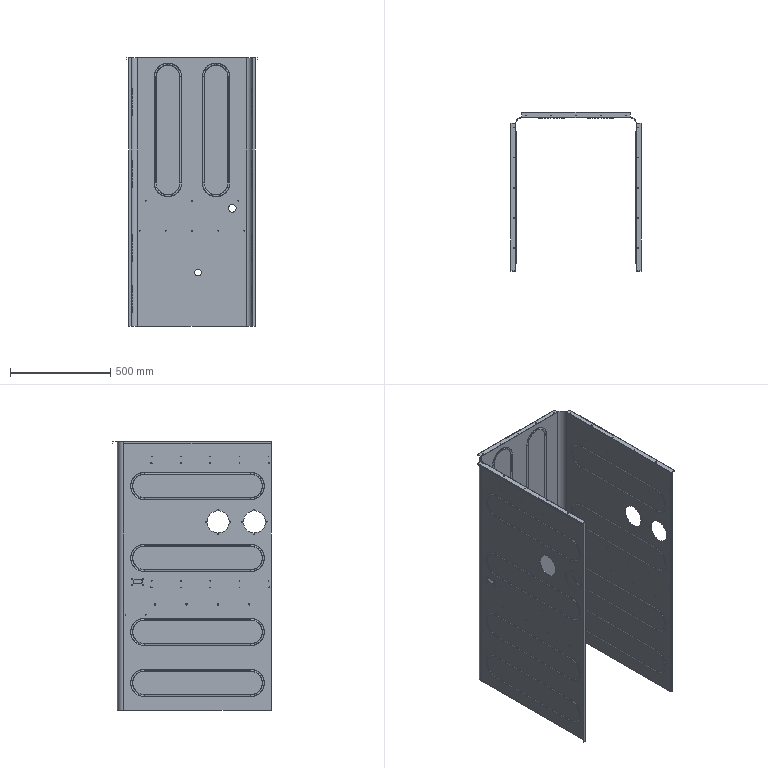Part | STEP file | HESS-408-70-15W-N-1-inner liner upper cover | 1 solid | 630 faces | box 650 x 790 x 1338 mm | volume 2883753 mm3 | cylinder 386 | spline 168 | plane 76 | commonest cylinder face diameters 2 x80 3.2 x64 3.5 x62 0.4 x40 2.4 x40 5.2 x24